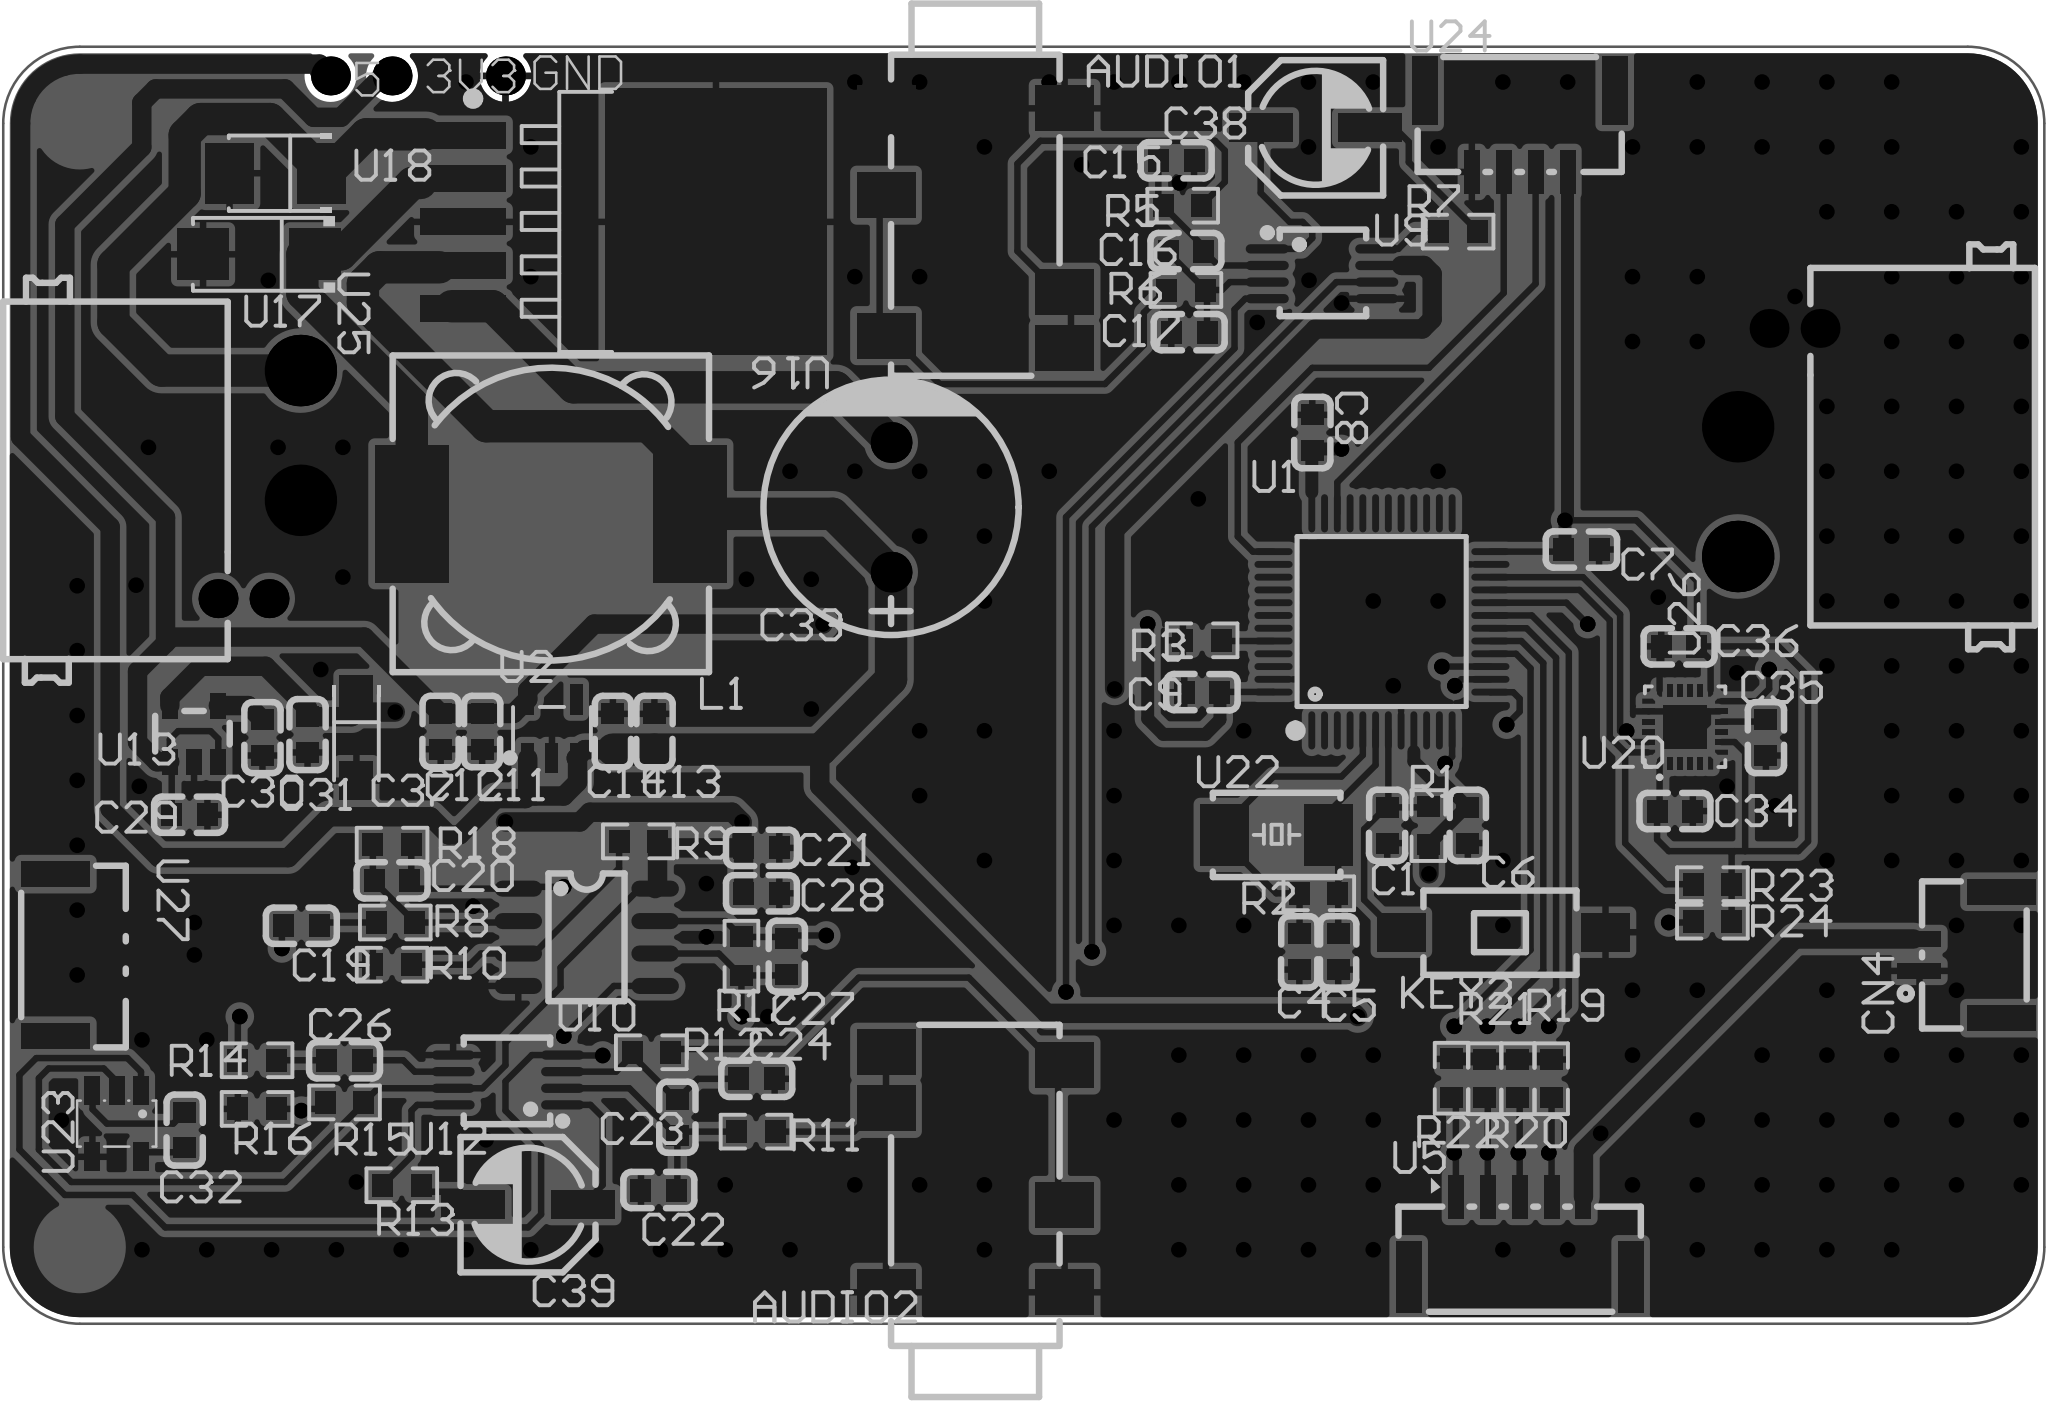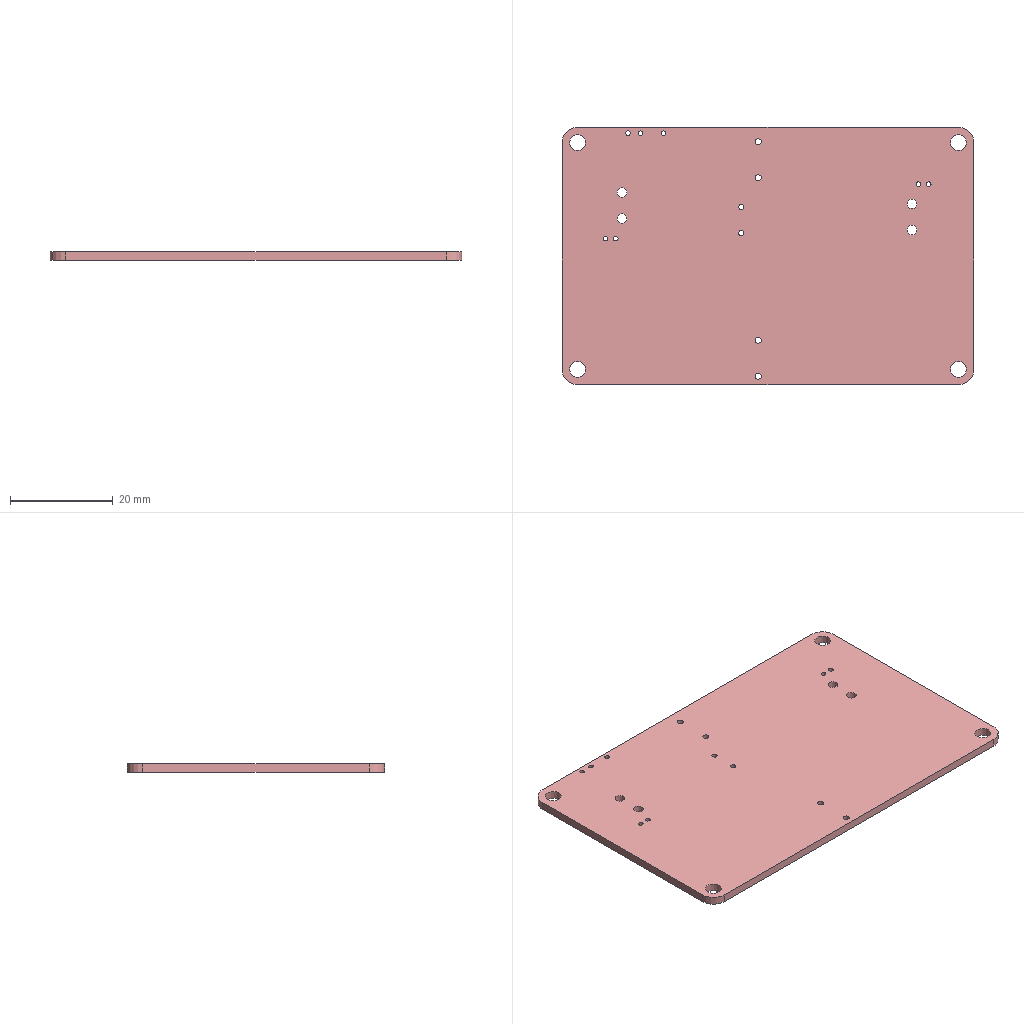Circuit board layout | Altium Designer | box 80 x 50 x 1.6 mm
Layer stack:
# Altium Designer layer stack of  (unit mm; dielectric type: 0 none, 1 core, 2 prepreg, 3 surface material)
index,name,kind,layer,copper_thickness_mm,dielectric_type,dielectric_thickness_mm,dielectric_material,dielectric_constant
0,Top Paste Mask Layer,other,,,,,,
1,Top Silkscreen Layer,other,,,,,,
2,Top Solder Mask Layer,dielectric,,,3,0.01,,3.3
3,Top Layer,copper,Top Layer,0.035,,,,
4,Dielectric1,dielectric,,,3,1.51,FR4,4.5
5,Bottom Layer,copper,Bottom Layer,0.035,,,,
6,Bottom Solder Mask Layer,dielectric,,,3,0.01,,3.3
7,Bottom Silkscreen Layer,other,,,,,,
8,Bottom Paste Mask Layer,other,,,,,,
# drill layer pairs: low layer,high layer
drill_pair,Top Layer,Bottom Layer
Part placement:
Designator,Comment,Layer,Footprint,Center-X(mm),Center-Y(mm),Rotation
R23,4.7K,TopLayer,R0603,147.382,100.179,180
R24,4.7K,TopLayer,R0603,147.382,98.713,180
C37,10uF,TopLayer,CAP-SMD_L3.2-W1.6-RD,94.234,105.918,270
U22,8MHz,TopLayer,OSC-SMD-2P_-L5.0-W3.2,130.302,102.108,0
CN4,GH1.25-2PWBPZ,TopLayer,CONN-SMD_GH1.25-2PWBPZ,157.099,97.409,90
AUDIO1,PJ-3420-A-SMT,TopLayer,AUDIO-SMD_PJ-3420-A-SMT_C319102,118.491,125.857,270
AUDIO2,PJ-3420-A-SMT,TopLayer,AUDIO-SMD_PJ-3420-A-SMT_C319102,118.491,88.9,90
C38,22uF,TopLayer,CAP-SMD_BD5.0-L5.3-W5.3-RD,131.826,129.794,180
C39,22uF,TopLayer,CAP-SMD_BD5.0-L5.3-W5.3-RD,100.965,87.63,0
C1,0.1u,TopLayer,C0603,134.637,102.488,90
C4,22pF,TopLayer,C0603,131.191,97.536,90
C5,22pF,TopLayer,C0603,132.715,97.536,90
C6,104,TopLayer,C0603,137.795,102.489,90
C7,104,TopLayer,C0603,142.24,113.284,180
C8,104,TopLayer,C0603,131.699,117.856,270
C9,104,TopLayer,C0603,127.381,107.696,0
C11,1uF,TopLayer,C0603,99.163,106.164,90
C12,0.1uF,TopLayer,C0603,97.536,106.164,90
C13,1uF,TopLayer,C0603,105.913,106.148,270
C14,0.1uF,TopLayer,C0603,104.286,106.148,270
C15,1nF,TopLayer,C0603,126.365,128.524,0
C16,1nF,TopLayer,C0603,126.746,124.968,0
C17,1nF,TopLayer,C0603,126.873,121.793,0
C19,1uF,TopLayer,C0603,92.075,98.552,180
C20,10nF,TopLayer,C0603,95.631,100.33,180
C21,100nF,TopLayer,C0603,110.109,101.6,0
C22,1nF,TopLayer,C0603,106.087,88.205,180
C23,1nF,TopLayer,C0603,106.813,91.055,270
C24,1nF,TopLayer,C0603,109.926,92.558,180
C26,1uF,TopLayer,C0603,93.768,93.285,0
C27,10nF,TopLayer,C0603,111.103,97.36,270
C28,100nF,TopLayer,C0603,110.109,99.822,0
C29,1uF,TopLayer,C0603,87.694,102.898,0
C30,470pF,TopLayer,C0603,90.551,105.918,270
C31,100nF,TopLayer,C0603,92.318,106.037,270
C32,1uF,TopLayer,C0603,87.503,90.551,90
C33,220uF,TopLayer,CAP-TH_BD10.0-P5.00-D1.0-FD,115.189,114.935,90
KEY2,TS-1101-C-W,TopLayer,SW-SMD_L6.0-W3.3-LS8.0,139.192,98.298,0
L1,47uH,TopLayer,IND-SMD_L12.3-W12.3,101.854,114.681,180
R1,10K,TopLayer,R0603,136.248,102.474,270
R2,1M,TopLayer,R0603,131.953,99.822,0
R3,10K,TopLayer,R0603,127.381,109.728,180
R5,0,TopLayer,R0603,126.619,126.746,180
R6,0,TopLayer,R0603,126.746,123.444,0
R7,300,TopLayer,R0603,137.414,125.73,180
R8,10K,TopLayer,R0603,95.758,98.679,0
R9,10K,TopLayer,R0603,105.283,101.854,180
R10,10K,TopLayer,R0603,95.631,97.028,0
R11,0,TopLayer,R0603,109.897,90.491,180
R12,0,TopLayer,R0603,105.791,93.599,180
R13,300,TopLayer,R0603,96.012,88.392,180
R14,10K,TopLayer,R0603,90.339,93.285,180
R15,10K,TopLayer,R0603,93.768,91.634,180
R16,10K,TopLayer,R0603,90.339,91.38,0
R17,24K,TopLayer,R0603,109.325,97.36,90
R18,24K,TopLayer,R0603,95.631,101.727,0
U1,STM32F103C8T6,TopLayer,LQFP-48_L7.0-W7.0-P0.50-LS9.0-BL,134.43,110.451,0
U2,ME6211C50M5G-N,TopLayer,SOT-23-5_L3.0-W1.7-P0.95-LS2.8-BL,101.899,106.267,0
U5,BX-GH1.25-5PWT,TopLayer,CONN-SMD_5P-P1.25_BX-GH1.25-5PWT,139.827,86.36,0
U9,INA333AIDGKR,TopLayer,MSOP-8_L3.0-W3.0-P0.65-LS5.0-BL,132.08,124.079,270
U10,LMV358IDT-P,TopLayer,SOP-8_L4.9-W3.9-P1.27-LS6.0-BL,103.26,98.1,270
U12,INA333AIDGKR,TopLayer,MSOP-8_L3.0-W3.0-P0.65-LS5.0-BL,100.17,92.514,90
U13,MIC5219-3.0YM5,TopLayer,SOT-23-5_L2.9-W1.6-P0.95-LS2.8-BL,87.87,106.073,0
U16,LM2596S-5.0,TopLayer,TO-263-5_L10.1-W8.7-P1.70-LS14.4-BR,103.378,126.111,180
U17,1N5822D_SMA,TopLayer,SMA_L4.3-W2.6-LS5.2-RD,90.424,124.841,180
U18,100uF,TopLayer,CAP-SMD_L3.5-W2.8-FD,91.059,128.016,180
R19,10K,TopLayer,R0603,141.059,92.562,270
R20,10K,TopLayer,R0603,139.759,92.562,270
R21,10K,TopLayer,R0603,138.46,92.562,270
R22,10K,TopLayer,R0603,137.16,92.583,270
U23,TPS60400DBVR,TopLayer,SOT-23-5_L3.0-W1.7-P0.95-LS2.8-BR,84.836,90.805,90
U24,GH1.25-4PWBPZ,TopLayer,CONN-SMD_GH1.25-4PWBPZ,139.827,129.667,0
U25,XT30PW(2+2)-M.G.B,TopLayer,CONN-TH_4P-XT30PW-M,90.424,115.824,270
U26,XT30PW(2+2)-M.G.B,TopLayer,CONN-TH_4P-XT30PW-M,149.987,117.475,90
U27,GH1.25-3PWBPZ,TopLayer,CONN-SMD_GH1.25-3PWBPZ,83.947,97.409,270
C34,10nF,TopLayer,C0603,145.913,103.043,0
C35,100nF,TopLayer,C0603,149.479,105.918,270
C36,100nF,TopLayer,C0603,146.076,109.49,180
U20,MPU-9250,TopLayer,QFN-24_L3.0-W3.0-P0.40-BL-EP,146.311,106.345,0
Pad and via stacks:
# Altium Designer via and pad stacks of  (unit mm). Each distinct definition once, with the count of objects using it.
# via: kind,start_layer,end_layer,hole_mm,diameter_mm,mode(0 simple;1 top-mid-bottom;2 full stack),diameter_per_layer,count,example_net
# pad: kind,layer,hole_mm,hole_type(0 round;1 square;2 slot),plating,top_size,top_shape(1 round;2 rect;3 octagon;9 rounded rect),mid_size,bottom_size,mode,footprint,size_per_layer,count,example
pad,Multi-Layer,0.9144,0,plated,1.524x1.524,1,1.524x1.524,1.524x1.524,0,,,3,1
pad,Multi-Layer,1,0,plated,1.6x1.6,1,1.6x1.6,1.6x1.6,0,CAP-TH_BD10.0-P5.00-D1.0-FD,,2,C33.1
pad,Multi-Layer,1.9,0,plated,2.8x2.8,1,2.8x2.8,2.8x2.8,0,CONN-TH_4P-XT30PW-M,,4,U25.1
pad,Multi-Layer,0.9144,0,plated,1.524x1.524,1,1.524x1.524,1.524x1.524,0,CONN-TH_4P-XT30PW-M,,4,U25.3
pad,Top Layer,0,0,plated,0.8065x0.864,2,0.8065x0.864,0.8065x0.864,0,R0603,,46,R23.2
pad,Top Layer,0,0,plated,1.5x1.296,2,1.5x1.296,1.5x1.296,0,CAP-SMD_L3.2-W1.6-RD,,2,C37.1
pad,Top Layer,0,0,plated,1.9x2.4,2,1.9x2.4,1.9x2.4,0,OSC-SMD-2P_-L5.0-W3.2,,2,U22.1
pad,Top Layer,0,0,plated,0.6x1.7,2,0.6x1.7,0.6x1.7,0,CONN-SMD_GH1.25-2PWBPZ,,2,CN4.1
pad,Top Layer,0,0,plated,1x2.7,2,1x2.7,1x2.7,0,CONN-SMD_GH1.25-2PWBPZ,,2,CN4.3
pad,Top Layer,0,0,plated,2.3x1.8,2,2.3x1.8,2.3x1.8,0,AUDIO-SMD_PJ-3420-A-SMT_C319102,,12,AUDIO1.1
pad,Top Layer,0,0,plated,2.5x1.1,2,2.5x1.1,2.5x1.1,0,CAP-SMD_BD5.0-L5.3-W5.3-RD,,4,C38.1
pad,Top Layer,0,0,plated,0.8x0.9,2,0.8x0.9,0.8x0.9,0,C0603,,60,C1.2
pad,Top Layer,0,0,plated,1.9x1.5,2,1.9x1.5,1.9x1.5,0,SW-SMD_L6.0-W3.3-LS8.0,,2,KEY2.1
pad,Top Layer,0,0,plated,2.9x5.4,2,2.9x5.4,2.9x5.4,0,IND-SMD_L12.3-W12.3,,2,L1.1
pad,Top Layer,0,0,plated,0.27x1.5,1,0.27x1.5,0.27x1.5,0,LQFP-48_L7.0-W7.0-P0.50-LS9.0-BL,,24,U1.1
pad,Top Layer,0,0,plated,1.5x0.27,1,1.5x0.27,1.5x0.27,0,LQFP-48_L7.0-W7.0-P0.50-LS9.0-BL,,24,U1.13
pad,Top Layer,0,0,plated,0.49x1.157,2,0.49x1.157,0.49x1.157,0,SOT-23-5_L3.0-W1.7-P0.95-LS2.8-BL,,3,U2.1
pad,Top Layer,0,0,plated,0.49x1.175,2,0.49x1.175,0.49x1.175,0,SOT-23-5_L3.0-W1.7-P0.95-LS2.8-BL,,2,U2.4
pad,Top Layer,0,0,plated,1x2.8,2,1x2.8,1x2.8,0,CONN-SMD_5P-P1.25_BX-GH1.25-5PWT,,2,U5.7
pad,Top Layer,0,0,plated,0.6x1.7,2,0.6x1.7,0.6x1.7,0,CONN-SMD_5P-P1.25_BX-GH1.25-5PWT,,5,U5.5
pad,Top Layer,0,0,plated,0.364x1.692,1,0.364x1.692,0.364x1.692,0,MSOP-8_L3.0-W3.0-P0.65-LS5.0-BL,,16,U9.1
pad,Top Layer,0,0,plated,0.63x1.865,1,0.63x1.865,0.63x1.865,0,SOP-8_L4.9-W3.9-P1.27-LS6.0-BL,,8,U10.1
pad,Top Layer,0,0,plated,0.6x1,2,0.6x1,0.6x1,0,SOT-23-5_L2.9-W1.6-P0.95-LS2.8-BL,,5,U13.5
pad,Top Layer,0,0,plated,8.7x10.431,2,8.7x10.431,8.7x10.431,0,TO-263-5_L10.1-W8.7-P1.70-LS14.4-BR,,1,U16.6
pad,Top Layer,0,0,plated,3.358x1.02,2,3.358x1.02,3.358x1.02,0,TO-263-5_L10.1-W8.7-P1.70-LS14.4-BR,,5,U16.5
pad,Top Layer,0,0,plated,2x2,2,2x2,2x2,0,SMA_L4.3-W2.6-LS5.2-RD,,2,U17.2
pad,Top Layer,0,0,plated,1.9x2.376,2,1.9x2.376,1.9x2.376,0,CAP-SMD_L3.5-W2.8-FD,,2,U18.2
pad,Top Layer,0,0,plated,1.1x0.6,2,1.1x0.6,1.1x0.6,0,SOT-23-5_L3.0-W1.7-P0.95-LS2.8-BR,,5,U23.5
pad,Top Layer,0,0,plated,0.6x1.7,2,0.6x1.7,0.6x1.7,0,CONN-SMD_GH1.25-4PWBPZ,,4,U24.1
pad,Top Layer,0,0,plated,1x2.7,2,1x2.7,1x2.7,0,CONN-SMD_GH1.25-4PWBPZ,,2,U24.5
pad,Top Layer,0,0,plated,0.6x1.8,2,0.6x1.8,0.6x1.8,0,CONN-SMD_GH1.25-3PWBPZ,,3,U27.3
pad,Top Layer,0,0,plated,1x2.7,2,1x2.7,1x2.7,0,CONN-SMD_GH1.25-3PWBPZ,,2,U27.4
pad,Top Layer,0,0,plated,0.2x0.505,2,0.2x0.505,0.2x0.505,0,QFN-24_L3.0-W3.0-P0.40-BL-EP,,8,U20.2
pad,Top Layer,0,0,plated,0.505x0.2,2,0.505x0.2,0.505x0.2,0,QFN-24_L3.0-W3.0-P0.40-BL-EP,,8,U20.8
pad,Top Layer,0,0,plated,0.0966x0.0966,1,0.0966x0.0966,0.0966x0.0966,0,QFN-24_L3.0-W3.0-P0.40-BL-EP,,4,U20.18
pad,Top Layer,0,0,plated,1.7x1.7,2,1.7x1.7,1.7x1.7,0,QFN-24_L3.0-W3.0-P0.40-BL-EP,,1,U20.25
pad,Top Layer,0,0,plated,0.0965x0.0965,1,0.0965x0.0965,0.0965x0.0965,0,QFN-24_L3.0-W3.0-P0.40-BL-EP,,4,U20.24
via,Top Layer,Bottom Layer,0.3048,0.61,0,,243,PB11
Copper pours:
name,layer,net,type(0 solid;1 hatched;2 none)
Top Layer-GND,Top Layer,GND,0
Bottom Layer-GND,Bottom Layer,GND,0
Design rules, without the lines most boards share:
# Altium Designer design rules of  (exported by Altium Designer, unit mm)
# columns: name | kind | enabled | priority | scope1 | scope2 | descriptor | typed fields (field=value)
Plane_innerPlane | 0 | disabled | 1 | All | All | Clearance Constraint (Gap=6mil) (Disabled)(All),(All) | gap=0.1524
Plane_innerPlane_1 | 63 | disabled | 1 | All | All | Board Clearance Constraint (Gap=0mil) (Disabled)(All) |
Copper_copperRegion | 0 | disabled | 2 | All | All | Clearance Constraint (Gap=6mil) (Disabled)(All),(All) | gap=0.1524
Copper_copperRegion_1 | 63 | disabled | 2 | All | All | Board Clearance Constraint (Gap=0mil) (Disabled)(All) |
safeClearance | 0 | enabled | 3 | All | All | Clearance Constraint (Gap=6mil) (All),(All) | gap=0.1524
safeClearance_1 | 63 | enabled | 3 | All | All | Board Clearance Constraint (Gap=0mil) (All) |
otherClearance | 52 | enabled | 1 | All | All | Hole To Hole Clearance (Gap=11.8mil) (All),(All) | gap=0.2997
trackWidth | 2 | enabled | 1 | All | All | Width Constraint (Min=5mil) (Max=100mil) (Preferred=10mil) (All) |
viaSize | 11 | enabled | 1 | All | All | Routing Via (MinHoleWidth=11.811mil) (MaxHoleWidth=236.22mil) (PreferredHoleWidth=12.008mil) (MinWidth=19.685mil) (MaxWidth=393.701mil) (PreferedWidth=24.016mil) (All) | via_min_hole=0.3 via_max_hole=6 via_preferred_diameter=0.61 via_preferred_hole=0.305